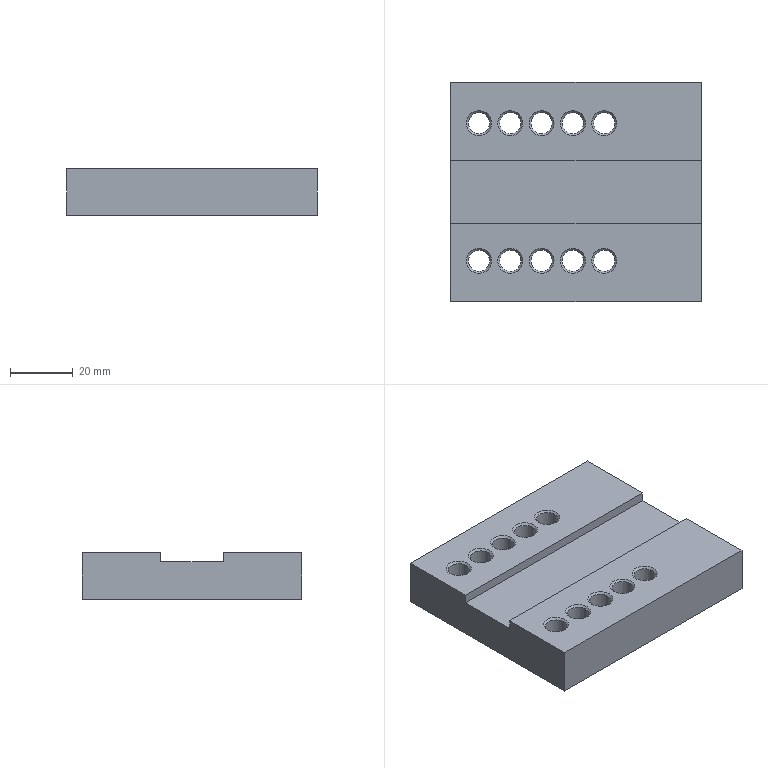Part | STEP file | Tube necking machine_id438_x_t | 1 solid | 40 faces | box 80 x 70 x 15 mm | volume 73671 mm3 | cone 20 | cylinder 10 | plane 10 | commonest cylinder face diameters 6.8 x10